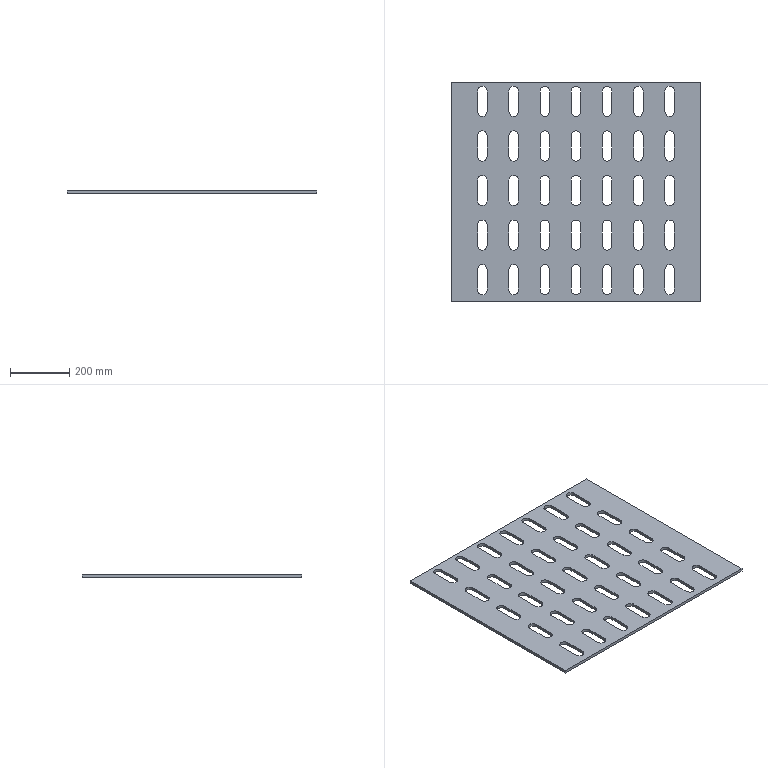Part | SolidWorks | features Extrusion 1, ICE 1 | 1 solid | 146 faces | box 840 x 740 x 10 mm | volume 5160574 mm3 | plane 76 | cylinder 70 | commonest cylinder face diameters 31.761 x70